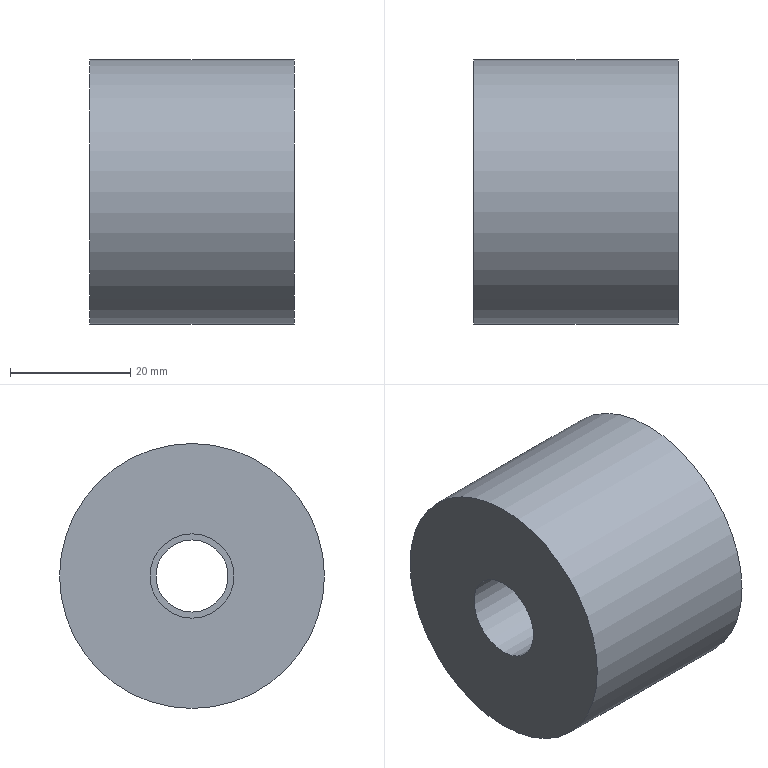Part | NX | 1 solid | 6 faces | box 34 x 44 x 44 mm | volume 47036 mm3 | cylinder 3 | plane 3 | commonest cylinder face diameters 12 x1 14 x1 44 x1
STEP:
#1=CARTESIAN_POINT('',(17.,0.,-6.));
#2=VERTEX_POINT('',#1);
#3=CARTESIAN_POINT('',(17.,0.,0.));
#4=DIRECTION('',(1.,0.,0.));
#5=DIRECTION('',(0.,0.,-1.));
#6=AXIS2_PLACEMENT_3D('',#3,#4,#5);
#7=CIRCLE('',#6,6.);
#8=EDGE_CURVE('',#2,#2,#7,.T.);
#9=ORIENTED_EDGE('',*,*,#8,.T.);
#10=EDGE_LOOP('',(#9));
#11=FACE_BOUND('',#10,.T.);
#12=CARTESIAN_POINT('',(3.,0.,6.));
#13=VERTEX_POINT('',#12);
#14=CARTESIAN_POINT('',(3.,0.,0.));
#15=DIRECTION('',(-1.,0.,0.));
#16=DIRECTION('',(0.,0.,1.));
#17=AXIS2_PLACEMENT_3D('',#14,#15,#16);
#18=CIRCLE('',#17,6.);
#19=EDGE_CURVE('',#13,#13,#18,.F.);
#20=ORIENTED_EDGE('',*,*,#19,.F.);
#21=EDGE_LOOP('',(#20));
#22=FACE_BOUND('',#21,.T.);
#23=CARTESIAN_POINT('',(-17.,0.,0.));
#24=DIRECTION('',(1.,0.,0.));
#25=DIRECTION('',(0.,0.,-1.));
#26=AXIS2_PLACEMENT_3D('',#23,#24,#25);
#27=CYLINDRICAL_SURFACE('',#26,6.);
#28=ADVANCED_FACE('',(#11,#22),#27,.F.);
#29=CARTESIAN_POINT('',(17.,0.,-22.));
#30=VERTEX_POINT('',#29);
#31=CARTESIAN_POINT('',(17.,0.,0.));
#32=DIRECTION('',(1.,0.,0.));
#33=DIRECTION('',(0.,0.,-1.));
#34=AXIS2_PLACEMENT_3D('',#31,#32,#33);
#35=CIRCLE('',#34,22.);
#36=EDGE_CURVE('',#30,#30,#35,.T.);
#37=ORIENTED_EDGE('',*,*,#36,.F.);
#38=EDGE_LOOP('',(#37));
#39=FACE_BOUND('',#38,.T.);
#40=CARTESIAN_POINT('',(-17.,0.,-22.));
#41=VERTEX_POINT('',#40);
#42=CARTESIAN_POINT('',(-17.,0.,0.));
#43=DIRECTION('',(1.,0.,0.));
#44=DIRECTION('',(0.,0.,-1.));
#45=AXIS2_PLACEMENT_3D('',#42,#43,#44);
#46=CIRCLE('',#45,22.);
#47=EDGE_CURVE('',#41,#41,#46,.T.);
#48=ORIENTED_EDGE('',*,*,#47,.T.);
#49=EDGE_LOOP('',(#48));
#50=FACE_BOUND('',#49,.T.);
#51=CARTESIAN_POINT('',(17.,0.,0.));
#52=DIRECTION('',(-1.,0.,0.));
#53=DIRECTION('',(0.,0.,1.));
#54=AXIS2_PLACEMENT_3D('',#51,#52,#53);
#55=CYLINDRICAL_SURFACE('',#54,22.);
#56=ADVANCED_FACE('',(#39,#50),#55,.T.);
#57=ORIENTED_EDGE('',*,*,#8,.F.);
#58=EDGE_LOOP('',(#57));
#59=FACE_BOUND('',#58,.T.);
#60=ORIENTED_EDGE('',*,*,#36,.T.);
#61=EDGE_LOOP('',(#60));
#62=FACE_BOUND('',#61,.T.);
#63=CARTESIAN_POINT('',(17.,0.,0.));
#64=DIRECTION('',(1.,0.,0.));
#65=DIRECTION('',(0.,0.,-1.));
#66=AXIS2_PLACEMENT_3D('',#63,#64,#65);
#67=PLANE('',#66);
#68=ADVANCED_FACE('',(#59,#62),#67,.T.);
#69=CARTESIAN_POINT('',(-17.,0.,7.));
#70=VERTEX_POINT('',#69);
#71=CARTESIAN_POINT('',(-17.,0.,0.));
#72=DIRECTION('',(-1.,0.,0.));
#73=DIRECTION('',(0.,0.,1.));
#74=AXIS2_PLACEMENT_3D('',#71,#72,#73);
#75=CIRCLE('',#74,7.);
#76=EDGE_CURVE('',#70,#70,#75,.T.);
#77=ORIENTED_EDGE('',*,*,#76,.F.);
#78=EDGE_LOOP('',(#77));
#79=FACE_BOUND('',#78,.T.);
#80=ORIENTED_EDGE('',*,*,#47,.F.);
#81=EDGE_LOOP('',(#80));
#82=FACE_BOUND('',#81,.T.);
#83=CARTESIAN_POINT('',(-17.,0.,0.));
#84=DIRECTION('',(1.,0.,0.));
#85=DIRECTION('',(0.,0.,-1.));
#86=AXIS2_PLACEMENT_3D('',#83,#84,#85);
#87=PLANE('',#86);
#88=ADVANCED_FACE('',(#79,#82),#87,.F.);
#89=CARTESIAN_POINT('',(3.,0.,7.));
#90=VERTEX_POINT('',#89);
#91=CARTESIAN_POINT('',(3.,0.,0.));
#92=DIRECTION('',(-1.,0.,0.));
#93=DIRECTION('',(0.,0.,1.));
#94=AXIS2_PLACEMENT_3D('',#91,#92,#93);
#95=CIRCLE('',#94,7.);
#96=EDGE_CURVE('',#90,#90,#95,.T.);
#97=ORIENTED_EDGE('',*,*,#96,.T.);
#98=EDGE_LOOP('',(#97));
#99=FACE_BOUND('',#98,.T.);
#100=ORIENTED_EDGE('',*,*,#19,.T.);
#101=EDGE_LOOP('',(#100));
#102=FACE_BOUND('',#101,.T.);
#103=CARTESIAN_POINT('',(3.,0.,0.));
#104=DIRECTION('',(-1.,0.,0.));
#105=DIRECTION('',(0.,0.,1.));
#106=AXIS2_PLACEMENT_3D('',#103,#104,#105);
#107=PLANE('',#106);
#108=ADVANCED_FACE('',(#99,#102),#107,.T.);
#109=ORIENTED_EDGE('',*,*,#96,.F.);
#110=EDGE_LOOP('',(#109));
#111=FACE_BOUND('',#110,.T.);
#112=ORIENTED_EDGE('',*,*,#76,.T.);
#113=EDGE_LOOP('',(#112));
#114=FACE_BOUND('',#113,.T.);
#115=CARTESIAN_POINT('',(3.,0.,0.));
#116=DIRECTION('',(-1.,0.,0.));
#117=DIRECTION('',(0.,0.,1.));
#118=AXIS2_PLACEMENT_3D('',#115,#116,#117);
#119=CYLINDRICAL_SURFACE('',#118,7.);
#120=ADVANCED_FACE('',(#111,#114),#119,.F.);
#121=CLOSED_SHELL('',(#28,#56,#68,#88,#108,#120));
#122=MANIFOLD_SOLID_BREP('',#121);
#123=(LENGTH_UNIT()NAMED_UNIT(*)SI_UNIT(.MILLI.,.METRE.));
#124=UNCERTAINTY_MEASURE_WITH_UNIT(LENGTH_MEASURE(0.00001),#123,'','');
#125=(NAMED_UNIT(*)PLANE_ANGLE_UNIT()SI_UNIT($,.RADIAN.));
#126=(NAMED_UNIT(*)SI_UNIT($,.STERADIAN.)SOLID_ANGLE_UNIT());
#127=(GEOMETRIC_REPRESENTATION_CONTEXT(3)GLOBAL_UNCERTAINTY_ASSIGNED_CONTEXT((#124))GLOBAL_UNIT_ASSIGNED_CONTEXT((#123,#125,#126))REPRESENTATION_CONTEXT('',''));
#128=ADVANCED_BREP_SHAPE_REPRESENTATION('',(#122),#127);